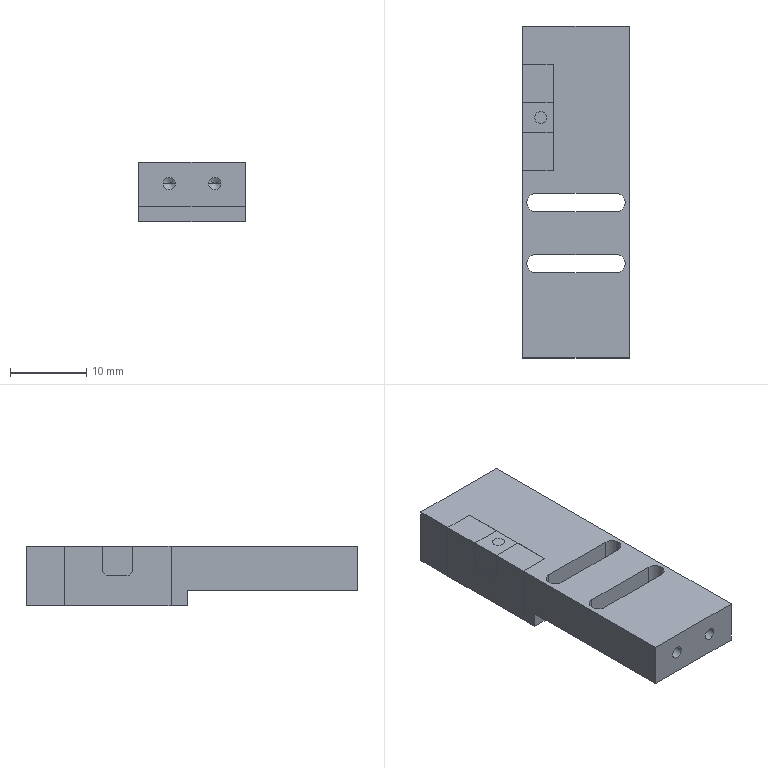NC program | NX | posted with a generic post | part box 14 x 43.5 x 7.8 mm
Whole program:
N10 G17 G21 G94 G90
(DRILLING , TOOL : D6A45)
N12 T07 M6
N14 G54
N16 G17 G0 G90 X0. Y1.9 B0. C0. S5000 M3
N18 G43 Z30. H7
N20 G94 G81 G98 Z-1. F250. R3.
N22 Y-2.1
N24 X-4. Y-0.1
N26 X4.
N28 G80
N30 G0 X4. Y-0.1 Z30.
N32 M5
(DRILLING_COPY_COPY , TOOL : 1.6ZT)
N34 T14 M6
N36 G54
N38 G17 G0 G90 X-4. Y-0.1 B0. C0. S2000 M3
N40 G43 Z30. H14
N42 G94 G83 G98 Z-4.2 F150. Q2. R3.
N44 X4.
N46 X0. Y1.9 Z-5.08
N48 Y-2.1
N50 G80
N52 G0 X0. Y-2.1 Z30.
N54 M5
(HOLE_MILLING_COPY , TOOL : D1.5)
N56 T13 M6
N58 G54
N60 G17 G0 G90 X0. Y1.9 B0. C0. S9500 M3
N62 G43 Z30. H13
N64 Z0.8
N66 G94 G3 X0.075 Y1.825 R0.075 F850.
N68 X0.15 Y1.9 R0.075
N70 X0.15 Y1.9 Z0.72 I-0.15 J0.
N72 X0.15 Y1.9 Z0.64 I-0.15 J0.
N74 X0.15 Y1.9 Z0.56 I-0.15 J0.
N76 X0.15 Y1.9 Z0.48 I-0.15 J0.
N78 X0.15 Y1.9 Z0.4 I-0.15 J0.
N80 X0.15 Y1.9 Z0.32 I-0.15 J0.
N82 X0.15 Y1.9 Z0.24 I-0.15 J0.
N84 X0.15 Y1.9 Z0.16 I-0.15 J0.
N86 X0.15 Y1.9 Z0.08 I-0.15 J0.
N88 X0.15 Y1.9 Z0. I-0.15 J0.
N90 X0.15 Y1.9 Z-0.08 I-0.15 J0.
N92 X0.15 Y1.9 Z-0.16 I-0.15 J0.
N94 X0.15 Y1.9 Z-0.24 I-0.15 J0.
N96 X0.15 Y1.9 Z-0.32 I-0.15 J0.
N98 X0.15 Y1.9 Z-0.4 I-0.15 J0.
N100 X0.15 Y1.9 Z-0.48 I-0.15 J0.
N102 X0.15 Y1.9 Z-0.56 I-0.15 J0.
N104 X0.15 Y1.9 Z-0.64 I-0.15 J0.
N106 X0.15 Y1.9 Z-0.72 I-0.15 J0.
N108 X0.15 Y1.9 Z-0.8 I-0.15 J0.
N110 X0.15 Y1.9 Z-0.88 I-0.15 J0.
N112 X0.15 Y1.9 Z-0.96 I-0.15 J0.
N114 X0.15 Y1.9 Z-1.04 I-0.15 J0.
N116 X0.15 Y1.9 Z-1.12 I-0.15 J0.
N118 X0.15 Y1.9 Z-1.2 I-0.15 J0.
N120 X0.15 Y1.9 Z-1.28 I-0.15 J0.
N122 X0.15 Y1.9 Z-1.36 I-0.15 J0.
N124 X0.15 Y1.9 Z-1.44 I-0.15 J0.
N126 X0.15 Y1.9 Z-1.52 I-0.15 J0.
N128 X0.15 Y1.9 Z-1.6 I-0.15 J0.
N130 X0.15 Y1.9 Z-1.68 I-0.15 J0.
N132 X0.15 Y1.9 Z-1.76 I-0.15 J0.
N134 X0.15 Y1.9 Z-1.84 I-0.15 J0.
N136 X0.15 Y1.9 Z-1.92 I-0.15 J0.
N138 X0.15 Y1.9 Z-2. I-0.15 J0.
N140 X0.15 Y1.9 Z-2.08 I-0.15 J0.
N142 X0.15 Y1.9 Z-2.16 I-0.15 J0.
N144 X0.15 Y1.9 Z-2.24 I-0.15 J0.
N146 X0.15 Y1.9 Z-2.32 I-0.15 J0.
N148 X0.15 Y1.9 Z-2.4 I-0.15 J0.
N150 X0.15 Y1.9 Z-2.48 I-0.15 J0.
N152 X0.15 Y1.9 Z-2.56 I-0.15 J0.
N154 X0.15 Y1.9 Z-2.64 I-0.15 J0.
N156 X0.15 Y1.9 Z-2.72 I-0.15 J0.
N158 X0.15 Y1.9 Z-2.8 I-0.15 J0.
N160 X0.15 Y1.9 Z-2.88 I-0.15 J0.
N162 X0.15 Y1.9 Z-2.96 I-0.15 J0.
N164 X0.15 Y1.9 Z-3.04 I-0.15 J0.
N166 X0.15 Y1.9 Z-3.12 I-0.15 J0.
N168 X0.15 Y1.9 Z-3.2 I-0.15 J0.
N170 X0.15 Y1.9 Z-3.28 I-0.15 J0.
N172 X0.15 Y1.9 Z-3.36 I-0.15 J0.
N174 X0.15 Y1.9 Z-3.44 I-0.15 J0.
N176 X0.15 Y1.9 Z-3.52 I-0.15 J0.
N178 X0.15 Y1.9 Z-3.6 I-0.15 J0.
N180 X0.15 Y1.9 Z-3.68 I-0.15 J0.
N182 X0.15 Y1.9 Z-3.76 I-0.15 J0.
N184 X0.15 Y1.9 Z-3.84 I-0.15 J0.
N186 X0.15 Y1.9 Z-3.92 I-0.15 J0.
N188 X0.15 Y1.9 Z-4. I-0.15 J0.
N190 X0.15 Y1.9 Z-4.08 I-0.15 J0.
N192 X0.15 Y1.9 Z-4.16 I-0.15 J0.
N194 X0.15 Y1.9 Z-4.24 I-0.15 J0.
N196 X0.15 Y1.9 Z-4.32 I-0.15 J0.
N198 X0.15 Y1.9 Z-4.4 I-0.15 J0.
N200 X0.15 Y1.9 Z-4.48 I-0.15 J0.
N202 X0.15 Y1.9 Z-4.56 I-0.15 J0.
N204 X-0.15 Y1.91 Z-4.599 R0.15
N206 X-0.01 Y1.75 R0.15
N208 X-0.15 Y1.91 R-0.15
N210 X-0.08 Y1.83 R0.075
N212 X0. Y1.9 R0.075
N214 G0 Z30.
N216 Y-2.1
N218 Z0.8
N220 G3 X0.075 Y-2.175 R0.075
N222 X0.15 Y-2.1 R0.075
N224 X0.15 Y-2.1 Z0.72 I-0.15 J0.
N226 X0.15 Y-2.1 Z0.64 I-0.15 J0.
N228 X0.15 Y-2.1 Z0.56 I-0.15 J0.
N230 X0.15 Y-2.1 Z0.48 I-0.15 J0.
N232 X0.15 Y-2.1 Z0.4 I-0.15 J0.
N234 X0.15 Y-2.1 Z0.32 I-0.15 J0.
N236 X0.15 Y-2.1 Z0.24 I-0.15 J0.
N238 X0.15 Y-2.1 Z0.16 I-0.15 J0.
N240 X0.15 Y-2.1 Z0.08 I-0.15 J0.
N242 X0.15 Y-2.1 Z0. I-0.15 J0.
N244 X0.15 Y-2.1 Z-0.08 I-0.15 J0.
N246 X0.15 Y-2.1 Z-0.16 I-0.15 J0.
N248 X0.15 Y-2.1 Z-0.24 I-0.15 J0.
N250 X0.15 Y-2.1 Z-0.32 I-0.15 J0.
N252 X0.15 Y-2.1 Z-0.4 I-0.15 J0.
N254 X0.15 Y-2.1 Z-0.48 I-0.15 J0.
N256 X0.15 Y-2.1 Z-0.56 I-0.15 J0.
N258 X0.15 Y-2.1 Z-0.64 I-0.15 J0.
N260 X0.15 Y-2.1 Z-0.72 I-0.15 J0.
N262 X0.15 Y-2.1 Z-0.8 I-0.15 J0.
N264 X0.15 Y-2.1 Z-0.88 I-0.15 J0.
N266 X0.15 Y-2.1 Z-0.96 I-0.15 J0.
N268 X0.15 Y-2.1 Z-1.04 I-0.15 J0.
N270 X0.15 Y-2.1 Z-1.12 I-0.15 J0.
N272 X0.15 Y-2.1 Z-1.2 I-0.15 J0.
N274 X0.15 Y-2.1 Z-1.28 I-0.15 J0.
N276 X0.15 Y-2.1 Z-1.36 I-0.15 J0.
N278 X0.15 Y-2.1 Z-1.44 I-0.15 J0.
N280 X0.15 Y-2.1 Z-1.52 I-0.15 J0.
N282 X0.15 Y-2.1 Z-1.6 I-0.15 J0.
N284 X0.15 Y-2.1 Z-1.68 I-0.15 J0.
N286 X0.15 Y-2.1 Z-1.76 I-0.15 J0.
N288 X0.15 Y-2.1 Z-1.84 I-0.15 J0.
N290 X0.15 Y-2.1 Z-1.92 I-0.15 J0.
N292 X0.15 Y-2.1 Z-2. I-0.15 J0.
N294 X0.15 Y-2.1 Z-2.08 I-0.15 J0.
N296 X0.15 Y-2.1 Z-2.16 I-0.15 J0.
N298 X0.15 Y-2.1 Z-2.24 I-0.15 J0.
N300 X0.15 Y-2.1 Z-2.32 I-0.15 J0.
N302 X0.15 Y-2.1 Z-2.4 I-0.15 J0.
N304 X0.15 Y-2.1 Z-2.48 I-0.15 J0.
N306 X0.15 Y-2.1 Z-2.56 I-0.15 J0.
N308 X0.15 Y-2.1 Z-2.64 I-0.15 J0.
N310 X0.15 Y-2.1 Z-2.72 I-0.15 J0.
N312 X0.15 Y-2.1 Z-2.8 I-0.15 J0.
N314 X0.15 Y-2.1 Z-2.88 I-0.15 J0.
N316 X0.15 Y-2.1 Z-2.96 I-0.15 J0.
N318 X0.15 Y-2.1 Z-3.04 I-0.15 J0.
N320 X0.15 Y-2.1 Z-3.12 I-0.15 J0.
N322 X0.15 Y-2.1 Z-3.2 I-0.15 J0.
N324 X0.15 Y-2.1 Z-3.28 I-0.15 J0.
N326 X0.15 Y-2.1 Z-3.36 I-0.15 J0.
N328 X0.15 Y-2.1 Z-3.44 I-0.15 J0.
N330 X0.15 Y-2.1 Z-3.52 I-0.15 J0.
N332 X0.15 Y-2.1 Z-3.6 I-0.15 J0.
N334 X0.15 Y-2.1 Z-3.68 I-0.15 J0.
N336 X0.15 Y-2.1 Z-3.76 I-0.15 J0.
N338 X0.15 Y-2.1 Z-3.84 I-0.15 J0.
N340 X0.15 Y-2.1 Z-3.92 I-0.15 J0.
N342 X0.15 Y-2.1 Z-4. I-0.15 J0.
N344 X0.15 Y-2.1 Z-4.08 I-0.15 J0.
N346 X0.15 Y-2.1 Z-4.16 I-0.15 J0.
N348 X0.15 Y-2.1 Z-4.24 I-0.15 J0.
N350 X0.15 Y-2.1 Z-4.32 I-0.15 J0.
N352 X0.15 Y-2.1 Z-4.4 I-0.15 J0.
N354 X0.15 Y-2.1 Z-4.48 I-0.15 J0.
N356 X0.15 Y-2.1 Z-4.56 I-0.15 J0.
N358 X-0.15 Y-2.09 Z-4.599 R0.15
N360 X-0.01 Y-2.25 R0.15
N362 X-0.15 Y-2.09 R-0.15
N364 X-0.08 Y-2.17 R0.075
N366 X0. Y-2.1 R0.075
N368 G0 Z30.
N370 M5
(DRILLING_COPY , TOOL : D6A45)
N372 T07 M6
N374 G54
N376 G17 G0 G90 X0. Y1.9 B0. C0. S5000 M3
N378 G43 Z30. H7
N380 G94 G81 G98 Z-1.15 F250. R3.
N382 Y-2.1
N384 G80
N386 G0 X0. Y-2.1 Z30.
N388 M5
(CUT_COMP_COPY , TOOL : D1.5)
N390 T13 M6
N392 G54
N394 G17 G0 G90 X0. Y1.9 B0. C0. S9500 M3
N396 G43 Z30. H13
N398 Z0.8
N400 G41 G94 G1 X0.065 Y1.824 F850. D13
N402 G3 X0.225 Y1.9 R0.098
N404 X0.225 Y1.9 Z0.3 I-0.225 J0.
N406 X0.225 Y1.9 Z-0.2 I-0.225 J0.
N408 X0.225 Y1.9 Z-0.7 I-0.225 J0.
N410 X0.225 Y1.9 Z-1.2 I-0.225 J0.
N412 X0.225 Y1.9 Z-1.7 I-0.225 J0.
N414 X0.225 Y1.9 Z-2.2 I-0.225 J0.
N416 X0.225 Y1.9 Z-2.7 I-0.225 J0.
N418 X0.225 Y1.9 Z-3.2 I-0.225 J0.
N420 X0.225 Y1.9 Z-3.7 I-0.225 J0.
N422 X0.225 Y1.9 Z-4.2 I-0.225 J0.
N424 X0.067 Y1.685 Z-4.599 R-0.225
N426 X0.215 Y1.967 R0.225
N428 X0.067 Y1.685 R-0.225
N430 X0.092 Y1.86 R0.098
N432 G40
N434 G1 X0. Y1.9
N436 G0 Z30.
N438 Y-2.1
N440 Z0.8
N442 G41 G1 X0.065 Y-2.176
N444 G3 X0.225 Y-2.1 R0.098
N446 X0.225 Y-2.1 Z0.3 I-0.225 J0.
N448 X0.225 Y-2.1 Z-0.2 I-0.225 J0.
N450 X0.225 Y-2.1 Z-0.7 I-0.225 J0.
N452 X0.225 Y-2.1 Z-1.2 I-0.225 J0.
N454 X0.225 Y-2.1 Z-1.7 I-0.225 J0.
N456 X0.225 Y-2.1 Z-2.2 I-0.225 J0.
N458 X0.225 Y-2.1 Z-2.7 I-0.225 J0.
N460 X0.225 Y-2.1 Z-3.2 I-0.225 J0.
N462 X0.225 Y-2.1 Z-3.7 I-0.225 J0.
N464 X0.225 Y-2.1 Z-4.2 I-0.225 J0.
N466 X0.067 Y-2.315 Z-4.599 R-0.225
N468 X0.215 Y-2.033 R0.225
N470 X0.067 Y-2.315 R-0.225
N472 X0.092 Y-2.14 R0.098
N474 G40
N476 G1 X0. Y-2.1
N478 G0 Z30.
N480 M5
N482 M2